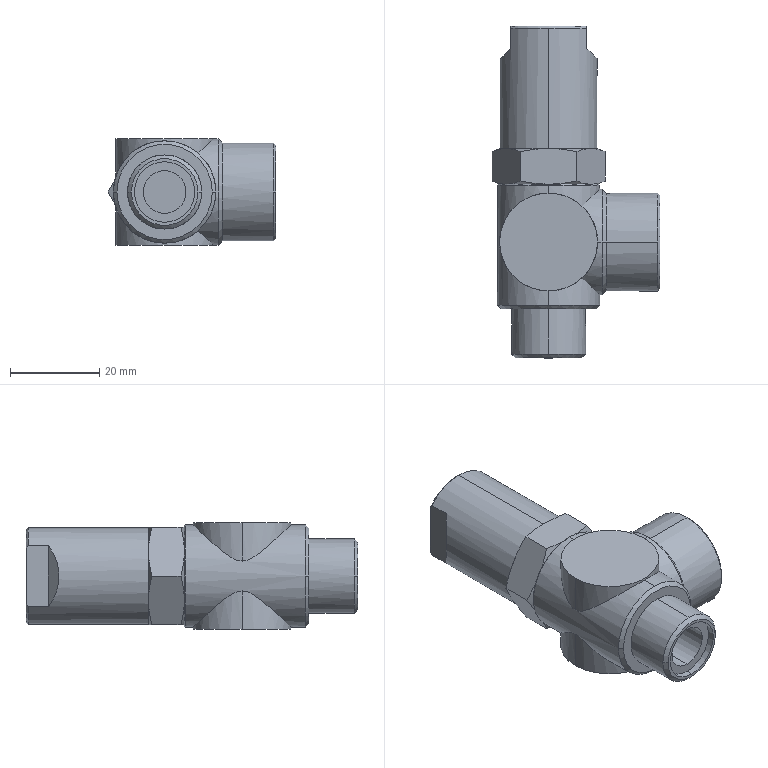Part | STEP file | PCV10 | 1 solid | 73 faces | box 37.702 x 74.5 x 24 mm | volume 30380 mm3 | cone 28 | cylinder 23 | plane 22 | commonest cylinder face diameters 22 x6 23 x3 9.602 x2 11.445 x2 13.602 x2 14.95 x2